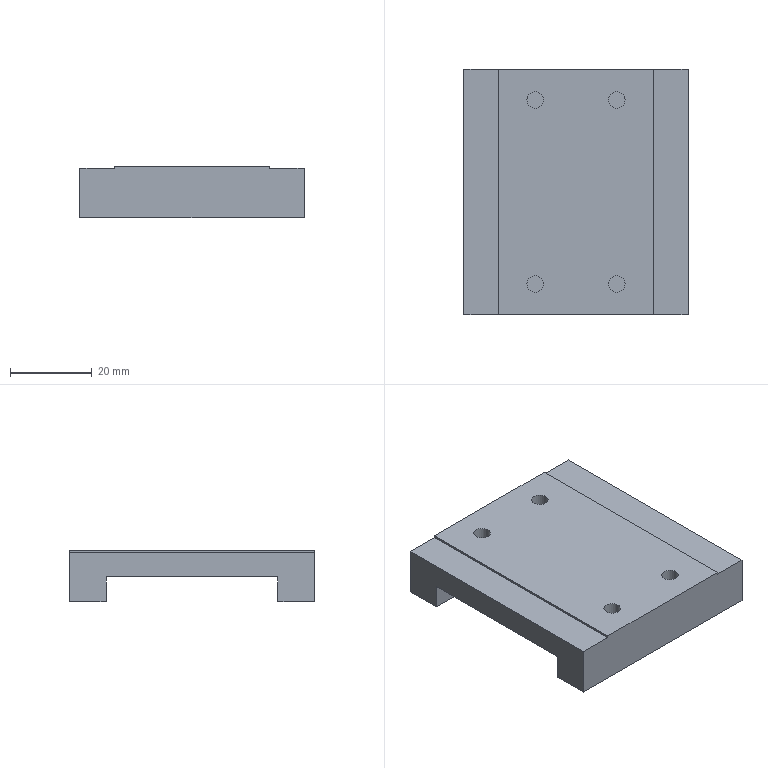Part | NX | features MGW_MGN15C00 2 | 1 solid | 22 faces | box 54.8 x 60 x 12.6 mm | volume 26674 mm3 | plane 18 | cylinder 4 | commonest cylinder face diameters 4 x4
STEP:
#1=CARTESIAN_POINT('',(68.173,47.5,11.8));
#2=VERTEX_POINT('',#1);
#3=CARTESIAN_POINT('',(66.173,47.5,11.8));
#4=DIRECTION('',(0.,0.,1.));
#5=DIRECTION('',(1.,0.,0.));
#6=AXIS2_PLACEMENT_3D('',#3,#4,#5);
#7=CIRCLE('',#6,2.);
#8=EDGE_CURVE('',#2,#2,#7,.T.);
#9=ORIENTED_EDGE('',*,*,#8,.T.);
#10=EDGE_LOOP('',(#9));
#11=FACE_BOUND('',#10,.T.);
#12=CARTESIAN_POINT('',(76.173,25.,11.8));
#13=DIRECTION('',(0.,0.,1.));
#14=DIRECTION('',(1.,0.,0.));
#15=AXIS2_PLACEMENT_3D('',#12,#13,#14);
#16=PLANE('',#15);
#17=ADVANCED_FACE('',(#11),#16,.T.);
#18=CARTESIAN_POINT('',(64.173,47.5,16.));
#19=VERTEX_POINT('',#18);
#20=CARTESIAN_POINT('',(66.173,47.5,16.));
#21=DIRECTION('',(0.,0.,-1.));
#22=DIRECTION('',(-1.,0.,0.));
#23=AXIS2_PLACEMENT_3D('',#20,#21,#22);
#24=CIRCLE('',#23,2.);
#25=EDGE_CURVE('',#19,#19,#24,.T.);
#26=ORIENTED_EDGE('',*,*,#25,.F.);
#27=EDGE_LOOP('',(#26));
#28=FACE_BOUND('',#27,.T.);
#29=ORIENTED_EDGE('',*,*,#8,.F.);
#30=EDGE_LOOP('',(#29));
#31=FACE_BOUND('',#30,.T.);
#32=CARTESIAN_POINT('',(66.173,47.5,6.143));
#33=DIRECTION('',(0.,0.,1.));
#34=DIRECTION('',(1.,0.,0.));
#35=AXIS2_PLACEMENT_3D('',#32,#33,#34);
#36=CYLINDRICAL_SURFACE('',#35,2.);
#37=ADVANCED_FACE('',(#28,#31),#36,.F.);
#38=CARTESIAN_POINT('',(88.173,47.5,11.8));
#39=VERTEX_POINT('',#38);
#40=CARTESIAN_POINT('',(86.173,47.5,11.8));
#41=DIRECTION('',(0.,0.,1.));
#42=DIRECTION('',(1.,0.,0.));
#43=AXIS2_PLACEMENT_3D('',#40,#41,#42);
#44=CIRCLE('',#43,2.);
#45=EDGE_CURVE('',#39,#39,#44,.T.);
#46=ORIENTED_EDGE('',*,*,#45,.T.);
#47=EDGE_LOOP('',(#46));
#48=FACE_BOUND('',#47,.T.);
#49=CARTESIAN_POINT('',(76.173,25.,11.8));
#50=DIRECTION('',(0.,0.,1.));
#51=DIRECTION('',(1.,0.,0.));
#52=AXIS2_PLACEMENT_3D('',#49,#50,#51);
#53=PLANE('',#52);
#54=ADVANCED_FACE('',(#48),#53,.T.);
#55=CARTESIAN_POINT('',(84.173,47.5,16.));
#56=VERTEX_POINT('',#55);
#57=CARTESIAN_POINT('',(86.173,47.5,16.));
#58=DIRECTION('',(0.,0.,-1.));
#59=DIRECTION('',(-1.,0.,0.));
#60=AXIS2_PLACEMENT_3D('',#57,#58,#59);
#61=CIRCLE('',#60,2.);
#62=EDGE_CURVE('',#56,#56,#61,.T.);
#63=ORIENTED_EDGE('',*,*,#62,.F.);
#64=EDGE_LOOP('',(#63));
#65=FACE_BOUND('',#64,.T.);
#66=ORIENTED_EDGE('',*,*,#45,.F.);
#67=EDGE_LOOP('',(#66));
#68=FACE_BOUND('',#67,.T.);
#69=CARTESIAN_POINT('',(86.173,47.5,6.143));
#70=DIRECTION('',(0.,0.,1.));
#71=DIRECTION('',(1.,0.,0.));
#72=AXIS2_PLACEMENT_3D('',#69,#70,#71);
#73=CYLINDRICAL_SURFACE('',#72,2.);
#74=ADVANCED_FACE('',(#65,#68),#73,.F.);
#75=CARTESIAN_POINT('',(88.173,2.5,11.8));
#76=VERTEX_POINT('',#75);
#77=CARTESIAN_POINT('',(86.173,2.5,11.8));
#78=DIRECTION('',(0.,0.,1.));
#79=DIRECTION('',(1.,0.,0.));
#80=AXIS2_PLACEMENT_3D('',#77,#78,#79);
#81=CIRCLE('',#80,2.);
#82=EDGE_CURVE('',#76,#76,#81,.T.);
#83=ORIENTED_EDGE('',*,*,#82,.T.);
#84=EDGE_LOOP('',(#83));
#85=FACE_BOUND('',#84,.T.);
#86=CARTESIAN_POINT('',(76.173,25.,11.8));
#87=DIRECTION('',(0.,0.,1.));
#88=DIRECTION('',(1.,0.,0.));
#89=AXIS2_PLACEMENT_3D('',#86,#87,#88);
#90=PLANE('',#89);
#91=ADVANCED_FACE('',(#85),#90,.T.);
#92=CARTESIAN_POINT('',(84.173,2.5,16.));
#93=VERTEX_POINT('',#92);
#94=CARTESIAN_POINT('',(86.173,2.5,16.));
#95=DIRECTION('',(0.,0.,-1.));
#96=DIRECTION('',(-1.,0.,0.));
#97=AXIS2_PLACEMENT_3D('',#94,#95,#96);
#98=CIRCLE('',#97,2.);
#99=EDGE_CURVE('',#93,#93,#98,.T.);
#100=ORIENTED_EDGE('',*,*,#99,.F.);
#101=EDGE_LOOP('',(#100));
#102=FACE_BOUND('',#101,.T.);
#103=ORIENTED_EDGE('',*,*,#82,.F.);
#104=EDGE_LOOP('',(#103));
#105=FACE_BOUND('',#104,.T.);
#106=CARTESIAN_POINT('',(86.173,2.5,6.143));
#107=DIRECTION('',(0.,0.,1.));
#108=DIRECTION('',(1.,0.,0.));
#109=AXIS2_PLACEMENT_3D('',#106,#107,#108);
#110=CYLINDRICAL_SURFACE('',#109,2.);
#111=ADVANCED_FACE('',(#102,#105),#110,.F.);
#112=CARTESIAN_POINT('',(103.573,-5.,15.5));
#113=VERTEX_POINT('',#112);
#114=CARTESIAN_POINT('',(103.573,55.,15.5));
#115=VERTEX_POINT('',#114);
#116=CARTESIAN_POINT('',(103.573,-5.,15.5));
#117=DIRECTION('',(0.,1.,0.));
#118=VECTOR('',#117,1000.);
#119=LINE('',#116,#118);
#120=EDGE_CURVE('',#113,#115,#119,.T.);
#121=ORIENTED_EDGE('',*,*,#120,.T.);
#122=CARTESIAN_POINT('',(95.173,55.,15.5));
#123=VERTEX_POINT('',#122);
#124=CARTESIAN_POINT('',(103.573,55.,15.5));
#125=DIRECTION('',(-1.,0.,0.));
#126=VECTOR('',#125,1000.);
#127=LINE('',#124,#126);
#128=EDGE_CURVE('',#115,#123,#127,.T.);
#129=ORIENTED_EDGE('',*,*,#128,.T.);
#130=CARTESIAN_POINT('',(95.173,-5.,15.5));
#131=VERTEX_POINT('',#130);
#132=CARTESIAN_POINT('',(95.173,-5.,15.5));
#133=DIRECTION('',(0.,1.,0.));
#134=VECTOR('',#133,1000.);
#135=LINE('',#132,#134);
#136=EDGE_CURVE('',#131,#123,#135,.T.);
#137=ORIENTED_EDGE('',*,*,#136,.F.);
#138=CARTESIAN_POINT('',(103.573,-5.,15.5));
#139=DIRECTION('',(-1.,0.,0.));
#140=VECTOR('',#139,1000.);
#141=LINE('',#138,#140);
#142=EDGE_CURVE('',#113,#131,#141,.T.);
#143=ORIENTED_EDGE('',*,*,#142,.F.);
#144=EDGE_LOOP('',(#121,#129,#137,#143));
#145=FACE_BOUND('',#144,.T.);
#146=CARTESIAN_POINT('',(103.573,55.,15.5));
#147=DIRECTION('',(0.,0.,-1.));
#148=DIRECTION('',(-1.,0.,0.));
#149=AXIS2_PLACEMENT_3D('',#146,#147,#148);
#150=PLANE('',#149);
#151=ADVANCED_FACE('',(#145),#150,.F.);
#152=CARTESIAN_POINT('',(48.773,46.,3.4));
#153=VERTEX_POINT('',#152);
#154=CARTESIAN_POINT('',(103.573,46.,3.4));
#155=VERTEX_POINT('',#154);
#156=CARTESIAN_POINT('',(48.773,46.,3.4));
#157=DIRECTION('',(1.,0.,0.));
#158=VECTOR('',#157,1000.);
#159=LINE('',#156,#158);
#160=EDGE_CURVE('',#153,#155,#159,.T.);
#161=ORIENTED_EDGE('',*,*,#160,.F.);
#162=CARTESIAN_POINT('',(48.773,55.,3.4));
#163=VERTEX_POINT('',#162);
#164=CARTESIAN_POINT('',(48.773,46.,3.4));
#165=DIRECTION('',(0.,1.,0.));
#166=VECTOR('',#165,1000.);
#167=LINE('',#164,#166);
#168=EDGE_CURVE('',#153,#163,#167,.T.);
#169=ORIENTED_EDGE('',*,*,#168,.T.);
#170=CARTESIAN_POINT('',(103.573,55.,3.4));
#171=VERTEX_POINT('',#170);
#172=CARTESIAN_POINT('',(48.773,55.,3.4));
#173=DIRECTION('',(1.,0.,0.));
#174=VECTOR('',#173,1000.);
#175=LINE('',#172,#174);
#176=EDGE_CURVE('',#163,#171,#175,.T.);
#177=ORIENTED_EDGE('',*,*,#176,.T.);
#178=CARTESIAN_POINT('',(103.573,55.,3.4));
#179=DIRECTION('',(0.,-1.,0.));
#180=VECTOR('',#179,1000.);
#181=LINE('',#178,#180);
#182=EDGE_CURVE('',#171,#155,#181,.T.);
#183=ORIENTED_EDGE('',*,*,#182,.T.);
#184=EDGE_LOOP('',(#161,#169,#177,#183));
#185=FACE_BOUND('',#184,.T.);
#186=CARTESIAN_POINT('',(48.773,55.,3.4));
#187=DIRECTION('',(0.,0.,1.));
#188=DIRECTION('',(1.,0.,0.));
#189=AXIS2_PLACEMENT_3D('',#186,#187,#188);
#190=PLANE('',#189);
#191=ADVANCED_FACE('',(#185),#190,.F.);
#192=CARTESIAN_POINT('',(48.773,46.,9.5));
#193=VERTEX_POINT('',#192);
#194=CARTESIAN_POINT('',(103.573,46.,9.5));
#195=VERTEX_POINT('',#194);
#196=CARTESIAN_POINT('',(48.773,46.,9.5));
#197=DIRECTION('',(1.,0.,0.));
#198=VECTOR('',#197,1000.);
#199=LINE('',#196,#198);
#200=EDGE_CURVE('',#193,#195,#199,.T.);
#201=ORIENTED_EDGE('',*,*,#200,.F.);
#202=CARTESIAN_POINT('',(48.773,46.,3.4));
#203=DIRECTION('',(0.,0.,1.));
#204=VECTOR('',#203,1000.);
#205=LINE('',#202,#204);
#206=EDGE_CURVE('',#153,#193,#205,.T.);
#207=ORIENTED_EDGE('',*,*,#206,.F.);
#208=ORIENTED_EDGE('',*,*,#160,.T.);
#209=CARTESIAN_POINT('',(103.573,46.,3.4));
#210=DIRECTION('',(0.,0.,1.));
#211=VECTOR('',#210,1000.);
#212=LINE('',#209,#211);
#213=EDGE_CURVE('',#155,#195,#212,.T.);
#214=ORIENTED_EDGE('',*,*,#213,.T.);
#215=EDGE_LOOP('',(#201,#207,#208,#214));
#216=FACE_BOUND('',#215,.T.);
#217=CARTESIAN_POINT('',(103.573,46.,9.5));
#218=DIRECTION('',(0.,1.,0.));
#219=DIRECTION('',(0.,0.,1.));
#220=AXIS2_PLACEMENT_3D('',#217,#218,#219);
#221=PLANE('',#220);
#222=ADVANCED_FACE('',(#216),#221,.F.);
#223=ORIENTED_EDGE('',*,*,#200,.T.);
#224=CARTESIAN_POINT('',(103.573,4.,9.5));
#225=VERTEX_POINT('',#224);
#226=CARTESIAN_POINT('',(103.573,46.,9.5));
#227=DIRECTION('',(0.,-1.,0.));
#228=VECTOR('',#227,1000.);
#229=LINE('',#226,#228);
#230=EDGE_CURVE('',#195,#225,#229,.T.);
#231=ORIENTED_EDGE('',*,*,#230,.T.);
#232=CARTESIAN_POINT('',(48.773,4.,9.5));
#233=VERTEX_POINT('',#232);
#234=CARTESIAN_POINT('',(48.773,4.,9.5));
#235=DIRECTION('',(1.,0.,0.));
#236=VECTOR('',#235,1000.);
#237=LINE('',#234,#236);
#238=EDGE_CURVE('',#233,#225,#237,.T.);
#239=ORIENTED_EDGE('',*,*,#238,.F.);
#240=CARTESIAN_POINT('',(48.773,46.,9.5));
#241=DIRECTION('',(0.,-1.,0.));
#242=VECTOR('',#241,1000.);
#243=LINE('',#240,#242);
#244=EDGE_CURVE('',#193,#233,#243,.T.);
#245=ORIENTED_EDGE('',*,*,#244,.F.);
#246=EDGE_LOOP('',(#223,#231,#239,#245));
#247=FACE_BOUND('',#246,.T.);
#248=CARTESIAN_POINT('',(103.573,4.,9.5));
#249=DIRECTION('',(0.,0.,1.));
#250=DIRECTION('',(1.,0.,0.));
#251=AXIS2_PLACEMENT_3D('',#248,#249,#250);
#252=PLANE('',#251);
#253=ADVANCED_FACE('',(#247),#252,.F.);
#254=ORIENTED_EDGE('',*,*,#238,.T.);
#255=CARTESIAN_POINT('',(103.573,4.,3.4));
#256=VERTEX_POINT('',#255);
#257=CARTESIAN_POINT('',(103.573,4.,9.5));
#258=DIRECTION('',(0.,0.,-1.));
#259=VECTOR('',#258,1000.);
#260=LINE('',#257,#259);
#261=EDGE_CURVE('',#225,#256,#260,.T.);
#262=ORIENTED_EDGE('',*,*,#261,.T.);
#263=CARTESIAN_POINT('',(48.773,4.,3.4));
#264=VERTEX_POINT('',#263);
#265=CARTESIAN_POINT('',(103.573,4.,3.4));
#266=DIRECTION('',(-1.,0.,0.));
#267=VECTOR('',#266,1000.);
#268=LINE('',#265,#267);
#269=EDGE_CURVE('',#256,#264,#268,.T.);
#270=ORIENTED_EDGE('',*,*,#269,.T.);
#271=CARTESIAN_POINT('',(48.773,4.,9.5));
#272=DIRECTION('',(0.,0.,-1.));
#273=VECTOR('',#272,1000.);
#274=LINE('',#271,#273);
#275=EDGE_CURVE('',#233,#264,#274,.T.);
#276=ORIENTED_EDGE('',*,*,#275,.F.);
#277=EDGE_LOOP('',(#254,#262,#270,#276));
#278=FACE_BOUND('',#277,.T.);
#279=CARTESIAN_POINT('',(103.573,4.,9.5));
#280=DIRECTION('',(0.,-1.,0.));
#281=DIRECTION('',(0.,0.,-1.));
#282=AXIS2_PLACEMENT_3D('',#279,#280,#281);
#283=PLANE('',#282);
#284=ADVANCED_FACE('',(#278),#283,.F.);
#285=ORIENTED_EDGE('',*,*,#269,.F.);
#286=CARTESIAN_POINT('',(103.573,-5.,3.4));
#287=VERTEX_POINT('',#286);
#288=CARTESIAN_POINT('',(103.573,4.,3.4));
#289=DIRECTION('',(0.,-1.,0.));
#290=VECTOR('',#289,1000.);
#291=LINE('',#288,#290);
#292=EDGE_CURVE('',#256,#287,#291,.T.);
#293=ORIENTED_EDGE('',*,*,#292,.T.);
#294=CARTESIAN_POINT('',(48.773,-5.,3.4));
#295=VERTEX_POINT('',#294);
#296=CARTESIAN_POINT('',(103.573,-5.,3.4));
#297=DIRECTION('',(-1.,0.,0.));
#298=VECTOR('',#297,1000.);
#299=LINE('',#296,#298);
#300=EDGE_CURVE('',#287,#295,#299,.T.);
#301=ORIENTED_EDGE('',*,*,#300,.T.);
#302=CARTESIAN_POINT('',(48.773,-5.,3.4));
#303=DIRECTION('',(0.,1.,0.));
#304=VECTOR('',#303,1000.);
#305=LINE('',#302,#304);
#306=EDGE_CURVE('',#295,#264,#305,.T.);
#307=ORIENTED_EDGE('',*,*,#306,.T.);
#308=EDGE_LOOP('',(#285,#293,#301,#307));
#309=FACE_BOUND('',#308,.T.);
#310=CARTESIAN_POINT('',(48.773,55.,3.4));
#311=DIRECTION('',(0.,0.,1.));
#312=DIRECTION('',(1.,0.,0.));
#313=AXIS2_PLACEMENT_3D('',#310,#311,#312);
#314=PLANE('',#313);
#315=ADVANCED_FACE('',(#309),#314,.F.);
#316=CARTESIAN_POINT('',(48.773,-5.,15.5));
#317=VERTEX_POINT('',#316);
#318=CARTESIAN_POINT('',(48.773,55.,15.5));
#319=VERTEX_POINT('',#318);
#320=CARTESIAN_POINT('',(48.773,-5.,15.5));
#321=DIRECTION('',(0.,1.,0.));
#322=VECTOR('',#321,1000.);
#323=LINE('',#320,#322);
#324=EDGE_CURVE('',#317,#319,#323,.T.);
#325=ORIENTED_EDGE('',*,*,#324,.T.);
#326=CARTESIAN_POINT('',(48.773,55.,3.4));
#327=DIRECTION('',(0.,0.,1.));
#328=VECTOR('',#327,1000.);
#329=LINE('',#326,#328);
#330=EDGE_CURVE('',#163,#319,#329,.T.);
#331=ORIENTED_EDGE('',*,*,#330,.F.);
#332=ORIENTED_EDGE('',*,*,#168,.F.);
#333=ORIENTED_EDGE('',*,*,#206,.T.);
#334=ORIENTED_EDGE('',*,*,#244,.T.);
#335=ORIENTED_EDGE('',*,*,#275,.T.);
#336=ORIENTED_EDGE('',*,*,#306,.F.);
#337=CARTESIAN_POINT('',(48.773,-5.,3.4));
#338=DIRECTION('',(0.,0.,1.));
#339=VECTOR('',#338,1000.);
#340=LINE('',#337,#339);
#341=EDGE_CURVE('',#295,#317,#340,.T.);
#342=ORIENTED_EDGE('',*,*,#341,.T.);
#343=EDGE_LOOP('',(#325,#331,#332,#333,#334,#335,#336,#342));
#344=FACE_BOUND('',#343,.T.);
#345=CARTESIAN_POINT('',(48.773,-5.,16.));
#346=DIRECTION('',(1.,0.,0.));
#347=DIRECTION('',(0.,0.,-1.));
#348=AXIS2_PLACEMENT_3D('',#345,#346,#347);
#349=PLANE('',#348);
#350=ADVANCED_FACE('',(#344),#349,.F.);
#351=CARTESIAN_POINT('',(57.173,-5.,15.5));
#352=VERTEX_POINT('',#351);
#353=CARTESIAN_POINT('',(57.173,55.,15.5));
#354=VERTEX_POINT('',#353);
#355=CARTESIAN_POINT('',(57.173,-5.,15.5));
#356=DIRECTION('',(0.,1.,0.));
#357=VECTOR('',#356,1000.);
#358=LINE('',#355,#357);
#359=EDGE_CURVE('',#352,#354,#358,.T.);
#360=ORIENTED_EDGE('',*,*,#359,.T.);
#361=CARTESIAN_POINT('',(57.173,55.,15.5));
#362=DIRECTION('',(-1.,0.,0.));
#363=VECTOR('',#362,1000.);
#364=LINE('',#361,#363);
#365=EDGE_CURVE('',#354,#319,#364,.T.);
#366=ORIENTED_EDGE('',*,*,#365,.T.);
#367=ORIENTED_EDGE('',*,*,#324,.F.);
#368=CARTESIAN_POINT('',(57.173,-5.,15.5));
#369=DIRECTION('',(-1.,0.,0.));
#370=VECTOR('',#369,1000.);
#371=LINE('',#368,#370);
#372=EDGE_CURVE('',#352,#317,#371,.T.);
#373=ORIENTED_EDGE('',*,*,#372,.F.);
#374=EDGE_LOOP('',(#360,#366,#367,#373));
#375=FACE_BOUND('',#374,.T.);
#376=CARTESIAN_POINT('',(48.773,55.,15.5));
#377=DIRECTION('',(0.,0.,-1.));
#378=DIRECTION('',(-1.,0.,0.));
#379=AXIS2_PLACEMENT_3D('',#376,#377,#378);
#380=PLANE('',#379);
#381=ADVANCED_FACE('',(#375),#380,.F.);
#382=CARTESIAN_POINT('',(57.173,-5.,16.));
#383=VERTEX_POINT('',#382);
#384=CARTESIAN_POINT('',(57.173,55.,16.));
#385=VERTEX_POINT('',#384);
#386=CARTESIAN_POINT('',(57.173,-5.,16.));
#387=DIRECTION('',(0.,1.,0.));
#388=VECTOR('',#387,1000.);
#389=LINE('',#386,#388);
#390=EDGE_CURVE('',#383,#385,#389,.T.);
#391=ORIENTED_EDGE('',*,*,#390,.T.);
#392=CARTESIAN_POINT('',(57.173,55.,16.));
#393=DIRECTION('',(0.,0.,-1.));
#394=VECTOR('',#393,1000.);
#395=LINE('',#392,#394);
#396=EDGE_CURVE('',#385,#354,#395,.T.);
#397=ORIENTED_EDGE('',*,*,#396,.T.);
#398=ORIENTED_EDGE('',*,*,#359,.F.);
#399=CARTESIAN_POINT('',(57.173,-5.,16.));
#400=DIRECTION('',(0.,0.,-1.));
#401=VECTOR('',#400,1000.);
#402=LINE('',#399,#401);
#403=EDGE_CURVE('',#383,#352,#402,.T.);
#404=ORIENTED_EDGE('',*,*,#403,.F.);
#405=EDGE_LOOP('',(#391,#397,#398,#404));
#406=FACE_BOUND('',#405,.T.);
#407=CARTESIAN_POINT('',(57.173,55.,16.));
#408=DIRECTION('',(1.,0.,0.));
#409=DIRECTION('',(0.,0.,-1.));
#410=AXIS2_PLACEMENT_3D('',#407,#408,#409);
#411=PLANE('',#410);
#412=ADVANCED_FACE('',(#406),#411,.F.);
#413=ORIENTED_EDGE('',*,*,#128,.F.);
#414=CARTESIAN_POINT('',(103.573,55.,3.4));
#415=DIRECTION('',(0.,0.,1.));
#416=VECTOR('',#415,1000.);
#417=LINE('',#414,#416);
#418=EDGE_CURVE('',#171,#115,#417,.T.);
#419=ORIENTED_EDGE('',*,*,#418,.F.);
#420=ORIENTED_EDGE('',*,*,#176,.F.);
#421=ORIENTED_EDGE('',*,*,#330,.T.);
#422=ORIENTED_EDGE('',*,*,#365,.F.);
#423=ORIENTED_EDGE('',*,*,#396,.F.);
#424=CARTESIAN_POINT('',(95.173,55.,16.));
#425=VERTEX_POINT('',#424);
#426=CARTESIAN_POINT('',(57.173,55.,16.));
#427=DIRECTION('',(1.,0.,0.));
#428=VECTOR('',#427,1000.);
#429=LINE('',#426,#428);
#430=EDGE_CURVE('',#385,#425,#429,.T.);
#431=ORIENTED_EDGE('',*,*,#430,.T.);
#432=CARTESIAN_POINT('',(95.173,55.,15.5));
#433=DIRECTION('',(0.,0.,1.));
#434=VECTOR('',#433,1000.);
#435=LINE('',#432,#434);
#436=EDGE_CURVE('',#123,#425,#435,.T.);
#437=ORIENTED_EDGE('',*,*,#436,.F.);
#438=EDGE_LOOP('',(#413,#419,#420,#421,#422,#423,#431,#437));
#439=FACE_BOUND('',#438,.T.);
#440=CARTESIAN_POINT('',(103.573,55.,16.));
#441=DIRECTION('',(0.,-1.,0.));
#442=DIRECTION('',(1.,0.,0.));
#443=AXIS2_PLACEMENT_3D('',#440,#441,#442);
#444=PLANE('',#443);
#445=ADVANCED_FACE('',(#439),#444,.F.);
#446=ORIENTED_EDGE('',*,*,#120,.F.);
#447=CARTESIAN_POINT('',(103.573,-5.,3.4));
#448=DIRECTION('',(0.,0.,1.));
#449=VECTOR('',#448,1000.);
#450=LINE('',#447,#449);
#451=EDGE_CURVE('',#287,#113,#450,.T.);
#452=ORIENTED_EDGE('',*,*,#451,.F.);
#453=ORIENTED_EDGE('',*,*,#292,.F.);
#454=ORIENTED_EDGE('',*,*,#261,.F.);
#455=ORIENTED_EDGE('',*,*,#230,.F.);
#456=ORIENTED_EDGE('',*,*,#213,.F.);
#457=ORIENTED_EDGE('',*,*,#182,.F.);
#458=ORIENTED_EDGE('',*,*,#418,.T.);
#459=EDGE_LOOP('',(#446,#452,#453,#454,#455,#456,#457,#458));
#460=FACE_BOUND('',#459,.T.);
#461=CARTESIAN_POINT('',(103.573,-5.,16.));
#462=DIRECTION('',(-1.,0.,0.));
#463=DIRECTION('',(0.,0.,1.));
#464=AXIS2_PLACEMENT_3D('',#461,#462,#463);
#465=PLANE('',#464);
#466=ADVANCED_FACE('',(#460),#465,.F.);
#467=ORIENTED_EDGE('',*,*,#142,.T.);
#468=CARTESIAN_POINT('',(95.173,-5.,16.));
#469=VERTEX_POINT('',#468);
#470=CARTESIAN_POINT('',(95.173,-5.,15.5));
#471=DIRECTION('',(0.,0.,1.));
#472=VECTOR('',#471,1000.);
#473=LINE('',#470,#472);
#474=EDGE_CURVE('',#131,#469,#473,.T.);
#475=ORIENTED_EDGE('',*,*,#474,.T.);
#476=CARTESIAN_POINT('',(95.173,-5.,16.));
#477=DIRECTION('',(-1.,0.,0.));
#478=VECTOR('',#477,1000.);
#479=LINE('',#476,#478);
#480=EDGE_CURVE('',#469,#383,#479,.T.);
#481=ORIENTED_EDGE('',*,*,#480,.T.);
#482=ORIENTED_EDGE('',*,*,#403,.T.);
#483=ORIENTED_EDGE('',*,*,#372,.T.);
#484=ORIENTED_EDGE('',*,*,#341,.F.);
#485=ORIENTED_EDGE('',*,*,#300,.F.);
#486=ORIENTED_EDGE('',*,*,#451,.T.);
#487=EDGE_LOOP('',(#467,#475,#481,#482,#483,#484,#485,#486));
#488=FACE_BOUND('',#487,.T.);
#489=CARTESIAN_POINT('',(103.573,-5.,16.));
#490=DIRECTION('',(0.,1.,0.));
#491=DIRECTION('',(-1.,0.,0.));
#492=AXIS2_PLACEMENT_3D('',#489,#490,#491);
#493=PLANE('',#492);
#494=ADVANCED_FACE('',(#488),#493,.F.);
#495=ORIENTED_EDGE('',*,*,#136,.T.);
#496=ORIENTED_EDGE('',*,*,#436,.T.);
#497=CARTESIAN_POINT('',(95.173,-5.,16.));
#498=DIRECTION('',(0.,1.,0.));
#499=VECTOR('',#498,1000.);
#500=LINE('',#497,#499);
#501=EDGE_CURVE('',#469,#425,#500,.T.);
#502=ORIENTED_EDGE('',*,*,#501,.F.);
#503=ORIENTED_EDGE('',*,*,#474,.F.);
#504=EDGE_LOOP('',(#495,#496,#502,#503));
#505=FACE_BOUND('',#504,.T.);
#506=CARTESIAN_POINT('',(95.173,55.,16.));
#507=DIRECTION('',(-1.,0.,0.));
#508=DIRECTION('',(0.,0.,1.));
#509=AXIS2_PLACEMENT_3D('',#506,#507,#508);
#510=PLANE('',#509);
#511=ADVANCED_FACE('',(#505),#510,.F.);
#512=ORIENTED_EDGE('',*,*,#25,.T.);
#513=EDGE_LOOP('',(#512));
#514=FACE_BOUND('',#513,.T.);
#515=ORIENTED_EDGE('',*,*,#62,.T.);
#516=EDGE_LOOP('',(#515));
#517=FACE_BOUND('',#516,.T.);
#518=ORIENTED_EDGE('',*,*,#99,.T.);
#519=EDGE_LOOP('',(#518));
#520=FACE_BOUND('',#519,.T.);
#521=CARTESIAN_POINT('',(68.173,2.5,16.));
#522=VERTEX_POINT('',#521);
#523=CARTESIAN_POINT('',(66.173,2.5,16.));
#524=DIRECTION('',(0.,0.,-1.));
#525=DIRECTION('',(1.,0.,0.));
#526=AXIS2_PLACEMENT_3D('',#523,#524,#525);
#527=CIRCLE('',#526,2.);
#528=EDGE_CURVE('',#522,#522,#527,.T.);
#529=ORIENTED_EDGE('',*,*,#528,.T.);
#530=EDGE_LOOP('',(#529));
#531=FACE_BOUND('',#530,.T.);
#532=ORIENTED_EDGE('',*,*,#430,.F.);
#533=ORIENTED_EDGE('',*,*,#390,.F.);
#534=ORIENTED_EDGE('',*,*,#480,.F.);
#535=ORIENTED_EDGE('',*,*,#501,.T.);
#536=EDGE_LOOP('',(#532,#533,#534,#535));
#537=FACE_BOUND('',#536,.T.);
#538=CARTESIAN_POINT('',(48.773,55.,16.));
#539=DIRECTION('',(0.,0.,1.));
#540=DIRECTION('',(1.,0.,0.));
#541=AXIS2_PLACEMENT_3D('',#538,#539,#540);
#542=PLANE('',#541);
#543=ADVANCED_FACE('',(#514,#517,#520,#531,#537),#542,.T.);
#544=CARTESIAN_POINT('',(64.173,2.5,11.8));
#545=VERTEX_POINT('',#544);
#546=CARTESIAN_POINT('',(66.173,2.5,11.8));
#547=DIRECTION('',(0.,0.,1.));
#548=DIRECTION('',(-1.,0.,0.));
#549=AXIS2_PLACEMENT_3D('',#546,#547,#548);
#550=CIRCLE('',#549,2.);
#551=EDGE_CURVE('',#545,#545,#550,.T.);
#552=ORIENTED_EDGE('',*,*,#551,.T.);
#553=EDGE_LOOP('',(#552));
#554=FACE_BOUND('',#553,.T.);
#555=CARTESIAN_POINT('',(76.173,25.,11.8));
#556=DIRECTION('',(0.,0.,1.));
#557=DIRECTION('',(1.,0.,0.));
#558=AXIS2_PLACEMENT_3D('',#555,#556,#557);
#559=PLANE('',#558);
#560=ADVANCED_FACE('',(#554),#559,.T.);
#561=ORIENTED_EDGE('',*,*,#528,.F.);
#562=EDGE_LOOP('',(#561));
#563=FACE_BOUND('',#562,.T.);
#564=ORIENTED_EDGE('',*,*,#551,.F.);
#565=EDGE_LOOP('',(#564));
#566=FACE_BOUND('',#565,.T.);
#567=CARTESIAN_POINT('',(66.173,2.5,6.143));
#568=DIRECTION('',(0.,0.,1.));
#569=DIRECTION('',(1.,0.,0.));
#570=AXIS2_PLACEMENT_3D('',#567,#568,#569);
#571=CYLINDRICAL_SURFACE('',#570,2.);
#572=ADVANCED_FACE('',(#563,#566),#571,.F.);
#573=CLOSED_SHELL('',(#17,#37,#54,#74,#91,#111,#151,#191,#222,#253,#284,#315,#350,#381,#412,#445,#466,#494,#511,#543,#560,#572));
#574=MANIFOLD_SOLID_BREP('',#573);
#575=(LENGTH_UNIT()NAMED_UNIT(*)SI_UNIT(.MILLI.,.METRE.));
#576=UNCERTAINTY_MEASURE_WITH_UNIT(LENGTH_MEASURE(0.00001),#575,'','');
#577=(NAMED_UNIT(*)PLANE_ANGLE_UNIT()SI_UNIT($,.RADIAN.));
#578=(NAMED_UNIT(*)SI_UNIT($,.STERADIAN.)SOLID_ANGLE_UNIT());
#579=(GEOMETRIC_REPRESENTATION_CONTEXT(3)GLOBAL_UNCERTAINTY_ASSIGNED_CONTEXT((#576))GLOBAL_UNIT_ASSIGNED_CONTEXT((#575,#577,#578))REPRESENTATION_CONTEXT('',''));
#580=ADVANCED_BREP_SHAPE_REPRESENTATION('',(#574),#579);